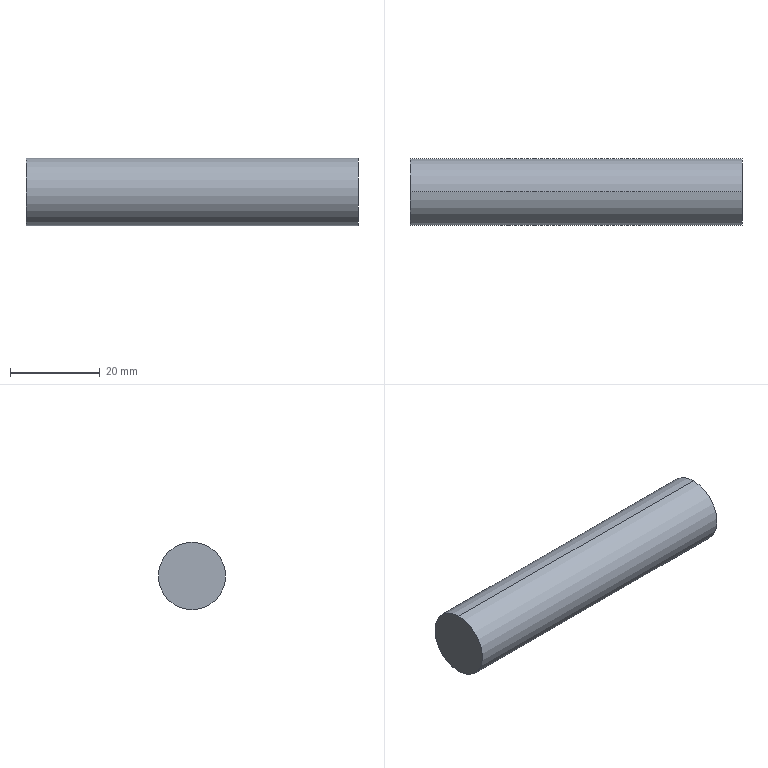Part | STEP file | PN_0015 (shaft rod) | 1 solid | 4 faces | box 74 x 15 x 15 mm | volume 13077 mm3 | cylinder 2 | plane 2 | commonest cylinder face diameters 15 x2
STEP:
#1=CARTESIAN_POINT('',(0.,0.,0.));
#2=DIRECTION('',(0.,0.,1.));
#3=DIRECTION('',(1.,0.,0.));
#4=AXIS2_PLACEMENT_3D('',#1,#2,#3);
#5=CARTESIAN_POINT('',(37.,0.,-7.5));
#6=VERTEX_POINT('',#5);
#7=CARTESIAN_POINT('',(37.,0.,7.5));
#8=VERTEX_POINT('',#7);
#9=CARTESIAN_POINT('',(37.,0.,0.));
#10=DIRECTION('',(1.,0.,0.));
#11=DIRECTION('',(0.,0.,-1.));
#12=AXIS2_PLACEMENT_3D('',#9,#10,#11);
#13=CIRCLE('',#12,7.5);
#14=CARTESIAN_POINT('',(37.,0.,0.));
#15=DIRECTION('',(-1.,0.,0.));
#16=DIRECTION('',(0.,0.,1.));
#17=AXIS2_PLACEMENT_3D('',#14,#15,#16);
#18=CYLINDRICAL_SURFACE('',#17,7.5);
#19=CARTESIAN_POINT('',(3.142,0.));
#20=DIRECTION('',(-1.,0.));
#21=VECTOR('',#20,1.);
#22=LINE('',#19,#21);
#23=(GEOMETRIC_REPRESENTATION_CONTEXT(2)PARAMETRIC_REPRESENTATION_CONTEXT()REPRESENTATION_CONTEXT('',''));
#24=DEFINITIONAL_REPRESENTATION('',(#22),#23);
#25=PCURVE('',#18,#24);
#26=CARTESIAN_POINT('',(37.,0.,0.));
#27=DIRECTION('',(1.,0.,0.));
#28=DIRECTION('',(0.,0.,-1.));
#29=AXIS2_PLACEMENT_3D('',#26,#27,#28);
#30=PLANE('',#29);
#31=CARTESIAN_POINT('',(0.,0.));
#32=DIRECTION('',(1.,0.));
#33=AXIS2_PLACEMENT_2D('',#31,#32);
#34=CIRCLE('',#33,7.5);
#35=(GEOMETRIC_REPRESENTATION_CONTEXT(2)PARAMETRIC_REPRESENTATION_CONTEXT()REPRESENTATION_CONTEXT('',''));
#36=DEFINITIONAL_REPRESENTATION('',(#34),#35);
#37=PCURVE('',#30,#36);
#38=SURFACE_CURVE('',#13,(#25,#37),.PCURVE_S1.);
#39=EDGE_CURVE('',#6,#8,#38,.T.);
#40=ORIENTED_EDGE('',*,*,#39,.F.);
#41=CARTESIAN_POINT('',(-37.,0.,-7.5));
#42=VERTEX_POINT('',#41);
#43=CARTESIAN_POINT('',(37.,0.,-7.5));
#44=DIRECTION('',(-1.,0.,0.));
#45=VECTOR('',#44,1.);
#46=LINE('',#43,#45);
#47=CARTESIAN_POINT('',(3.142,0.));
#48=DIRECTION('',(0.,1.));
#49=VECTOR('',#48,1.);
#50=LINE('',#47,#49);
#51=(GEOMETRIC_REPRESENTATION_CONTEXT(2)PARAMETRIC_REPRESENTATION_CONTEXT()REPRESENTATION_CONTEXT('',''));
#52=DEFINITIONAL_REPRESENTATION('',(#50),#51);
#53=PCURVE('',#18,#52);
#54=CARTESIAN_POINT('',(37.,0.,0.));
#55=DIRECTION('',(-1.,0.,0.));
#56=DIRECTION('',(0.,0.,1.));
#57=AXIS2_PLACEMENT_3D('',#54,#55,#56);
#58=CYLINDRICAL_SURFACE('',#57,7.5);
#59=CARTESIAN_POINT('',(3.142,0.));
#60=DIRECTION('',(0.,1.));
#61=VECTOR('',#60,1.);
#62=LINE('',#59,#61);
#63=(GEOMETRIC_REPRESENTATION_CONTEXT(2)PARAMETRIC_REPRESENTATION_CONTEXT()REPRESENTATION_CONTEXT('',''));
#64=DEFINITIONAL_REPRESENTATION('',(#62),#63);
#65=PCURVE('',#58,#64);
#66=SURFACE_CURVE('',#46,(#53,#65),.PCURVE_S1.);
#67=EDGE_CURVE('',#6,#42,#66,.T.);
#68=ORIENTED_EDGE('',*,*,#67,.T.);
#69=CARTESIAN_POINT('',(-37.,0.,7.5));
#70=VERTEX_POINT('',#69);
#71=CARTESIAN_POINT('',(-37.,0.,0.));
#72=DIRECTION('',(1.,0.,0.));
#73=DIRECTION('',(0.,0.,-1.));
#74=AXIS2_PLACEMENT_3D('',#71,#72,#73);
#75=CIRCLE('',#74,7.5);
#76=CARTESIAN_POINT('',(3.142,74.));
#77=DIRECTION('',(-1.,0.));
#78=VECTOR('',#77,1.);
#79=LINE('',#76,#78);
#80=(GEOMETRIC_REPRESENTATION_CONTEXT(2)PARAMETRIC_REPRESENTATION_CONTEXT()REPRESENTATION_CONTEXT('',''));
#81=DEFINITIONAL_REPRESENTATION('',(#79),#80);
#82=PCURVE('',#18,#81);
#83=CARTESIAN_POINT('',(-37.,0.,0.));
#84=DIRECTION('',(1.,0.,0.));
#85=DIRECTION('',(0.,0.,-1.));
#86=AXIS2_PLACEMENT_3D('',#83,#84,#85);
#87=PLANE('',#86);
#88=CARTESIAN_POINT('',(0.,0.));
#89=DIRECTION('',(1.,0.));
#90=AXIS2_PLACEMENT_2D('',#88,#89);
#91=CIRCLE('',#90,7.5);
#92=(GEOMETRIC_REPRESENTATION_CONTEXT(2)PARAMETRIC_REPRESENTATION_CONTEXT()REPRESENTATION_CONTEXT('',''));
#93=DEFINITIONAL_REPRESENTATION('',(#91),#92);
#94=PCURVE('',#87,#93);
#95=SURFACE_CURVE('',#75,(#82,#94),.PCURVE_S1.);
#96=EDGE_CURVE('',#42,#70,#95,.T.);
#97=ORIENTED_EDGE('',*,*,#96,.T.);
#98=CARTESIAN_POINT('',(37.,0.,7.5));
#99=DIRECTION('',(-1.,0.,0.));
#100=VECTOR('',#99,1.);
#101=LINE('',#98,#100);
#102=CARTESIAN_POINT('',(0.,0.));
#103=DIRECTION('',(0.,1.));
#104=VECTOR('',#103,1.);
#105=LINE('',#102,#104);
#106=(GEOMETRIC_REPRESENTATION_CONTEXT(2)PARAMETRIC_REPRESENTATION_CONTEXT()REPRESENTATION_CONTEXT('',''));
#107=DEFINITIONAL_REPRESENTATION('',(#105),#106);
#108=PCURVE('',#18,#107);
#109=CARTESIAN_POINT('',(6.283,0.));
#110=DIRECTION('',(0.,1.));
#111=VECTOR('',#110,1.);
#112=LINE('',#109,#111);
#113=(GEOMETRIC_REPRESENTATION_CONTEXT(2)PARAMETRIC_REPRESENTATION_CONTEXT()REPRESENTATION_CONTEXT('',''));
#114=DEFINITIONAL_REPRESENTATION('',(#112),#113);
#115=PCURVE('',#58,#114);
#116=SURFACE_CURVE('',#101,(#108,#115),.PCURVE_S1.);
#117=EDGE_CURVE('',#8,#70,#116,.T.);
#118=ORIENTED_EDGE('',*,*,#117,.F.);
#119=EDGE_LOOP('',(#40,#68,#97,#118));
#120=FACE_BOUND('',#119,.T.);
#121=ADVANCED_FACE('',(#120),#18,.T.);
#122=ORIENTED_EDGE('',*,*,#67,.F.);
#123=CARTESIAN_POINT('',(37.,0.,0.));
#124=DIRECTION('',(1.,0.,0.));
#125=DIRECTION('',(0.,0.,-1.));
#126=AXIS2_PLACEMENT_3D('',#123,#124,#125);
#127=CIRCLE('',#126,7.5);
#128=CARTESIAN_POINT('',(9.425,0.));
#129=DIRECTION('',(-1.,0.));
#130=VECTOR('',#129,1.);
#131=LINE('',#128,#130);
#132=(GEOMETRIC_REPRESENTATION_CONTEXT(2)PARAMETRIC_REPRESENTATION_CONTEXT()REPRESENTATION_CONTEXT('',''));
#133=DEFINITIONAL_REPRESENTATION('',(#131),#132);
#134=PCURVE('',#58,#133);
#135=CARTESIAN_POINT('',(0.,0.));
#136=DIRECTION('',(1.,0.));
#137=AXIS2_PLACEMENT_2D('',#135,#136);
#138=CIRCLE('',#137,7.5);
#139=(GEOMETRIC_REPRESENTATION_CONTEXT(2)PARAMETRIC_REPRESENTATION_CONTEXT()REPRESENTATION_CONTEXT('',''));
#140=DEFINITIONAL_REPRESENTATION('',(#138),#139);
#141=PCURVE('',#30,#140);
#142=SURFACE_CURVE('',#127,(#134,#141),.PCURVE_S1.);
#143=EDGE_CURVE('',#8,#6,#142,.T.);
#144=ORIENTED_EDGE('',*,*,#143,.F.);
#145=ORIENTED_EDGE('',*,*,#117,.T.);
#146=CARTESIAN_POINT('',(-37.,0.,0.));
#147=DIRECTION('',(1.,0.,0.));
#148=DIRECTION('',(0.,0.,-1.));
#149=AXIS2_PLACEMENT_3D('',#146,#147,#148);
#150=CIRCLE('',#149,7.5);
#151=CARTESIAN_POINT('',(9.425,74.));
#152=DIRECTION('',(-1.,0.));
#153=VECTOR('',#152,1.);
#154=LINE('',#151,#153);
#155=(GEOMETRIC_REPRESENTATION_CONTEXT(2)PARAMETRIC_REPRESENTATION_CONTEXT()REPRESENTATION_CONTEXT('',''));
#156=DEFINITIONAL_REPRESENTATION('',(#154),#155);
#157=PCURVE('',#58,#156);
#158=CARTESIAN_POINT('',(0.,0.));
#159=DIRECTION('',(1.,0.));
#160=AXIS2_PLACEMENT_2D('',#158,#159);
#161=CIRCLE('',#160,7.5);
#162=(GEOMETRIC_REPRESENTATION_CONTEXT(2)PARAMETRIC_REPRESENTATION_CONTEXT()REPRESENTATION_CONTEXT('',''));
#163=DEFINITIONAL_REPRESENTATION('',(#161),#162);
#164=PCURVE('',#87,#163);
#165=SURFACE_CURVE('',#150,(#157,#164),.PCURVE_S1.);
#166=EDGE_CURVE('',#70,#42,#165,.T.);
#167=ORIENTED_EDGE('',*,*,#166,.T.);
#168=EDGE_LOOP('',(#122,#144,#145,#167));
#169=FACE_BOUND('',#168,.T.);
#170=ADVANCED_FACE('',(#169),#58,.T.);
#171=ORIENTED_EDGE('',*,*,#143,.T.);
#172=ORIENTED_EDGE('',*,*,#39,.T.);
#173=EDGE_LOOP('',(#171,#172));
#174=FACE_BOUND('',#173,.T.);
#175=ADVANCED_FACE('',(#174),#30,.T.);
#176=ORIENTED_EDGE('',*,*,#166,.F.);
#177=ORIENTED_EDGE('',*,*,#96,.F.);
#178=EDGE_LOOP('',(#176,#177));
#179=FACE_BOUND('',#178,.T.);
#180=ADVANCED_FACE('',(#179),#87,.F.);
#181=CLOSED_SHELL('',(#121,#170,#175,#180));
#182=MANIFOLD_SOLID_BREP('',#181);
#183=(LENGTH_UNIT()NAMED_UNIT(*)SI_UNIT(.MILLI.,.METRE.));
#184=UNCERTAINTY_MEASURE_WITH_UNIT(LENGTH_MEASURE(0.0000001),#183,'','');
#185=(NAMED_UNIT(*)PLANE_ANGLE_UNIT()SI_UNIT($,.RADIAN.));
#186=(NAMED_UNIT(*)SI_UNIT($,.STERADIAN.)SOLID_ANGLE_UNIT());
#187=(GEOMETRIC_REPRESENTATION_CONTEXT(3)GLOBAL_UNCERTAINTY_ASSIGNED_CONTEXT((#184))GLOBAL_UNIT_ASSIGNED_CONTEXT((#183,#185,#186))REPRESENTATION_CONTEXT('',''));
#188=ADVANCED_BREP_SHAPE_REPRESENTATION('',(#4,#182),#187);